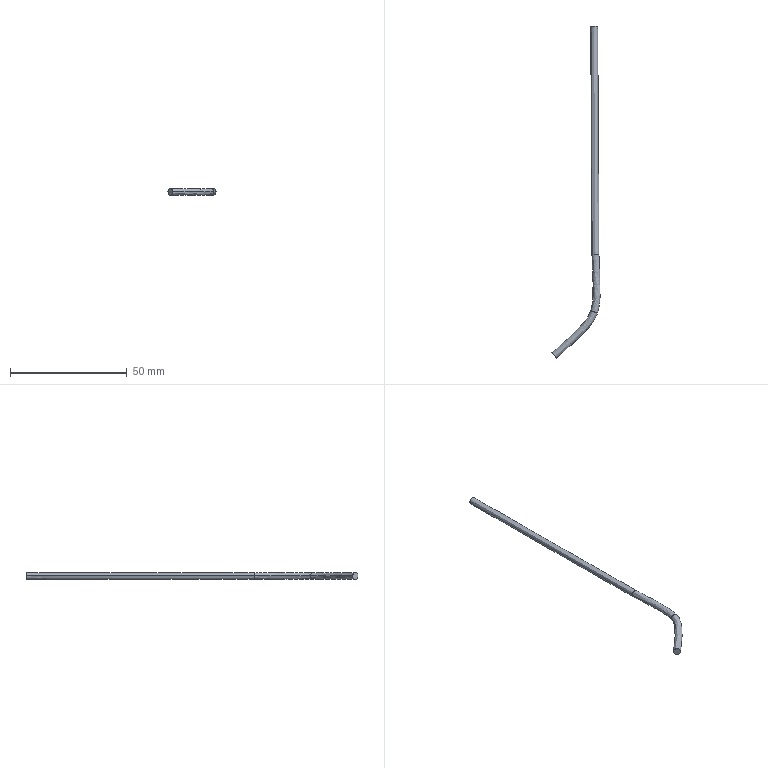Part | NX | features BREP 1 | 1 solid | 8 faces | box 20.654 x 142.358 x 3 mm | volume 1047 mm3 | spline 6 | plane 2